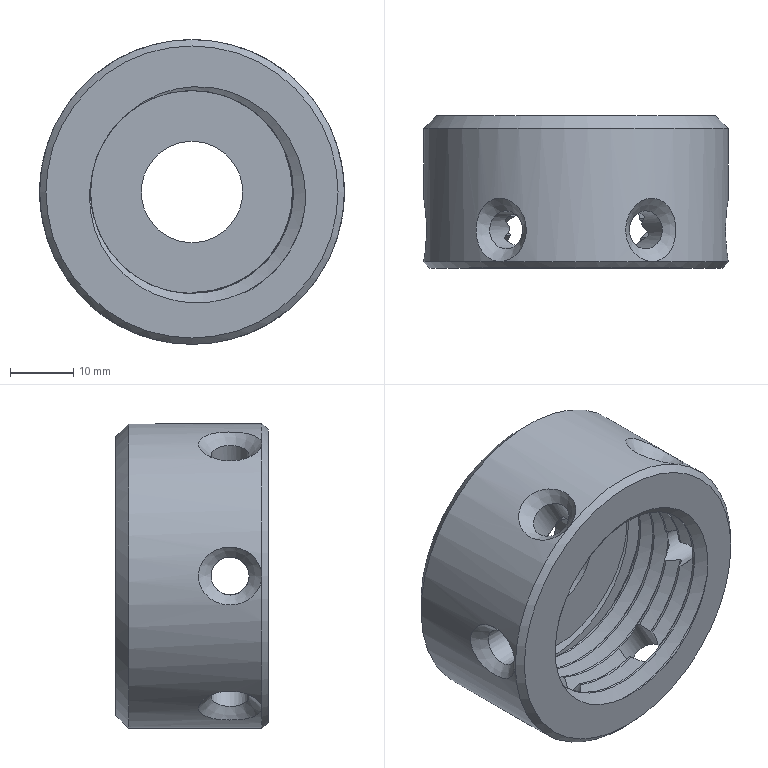Part | NX | features DATUM_CSYS 8, SKETCH 7, SWP104 7, EXTRACT_DATUM_AXIS 6, EXTRACT_DATUM_PLANE 6, EXTRACT_FACE 6, Instance Feature 5, CHAMFER 2, DATUM_PLANE 1, Pattern Feature 1, THREADS 1 | 1 solid | 70 faces | box 48 x 24 x 48 mm | volume 25018 mm3 | cylinder 35 | spline 22 | cone 8 | plane 5 | commonest cylinder face diameters 32 x13 36 x13 6 x6 16 x1 38 x1 48 x1